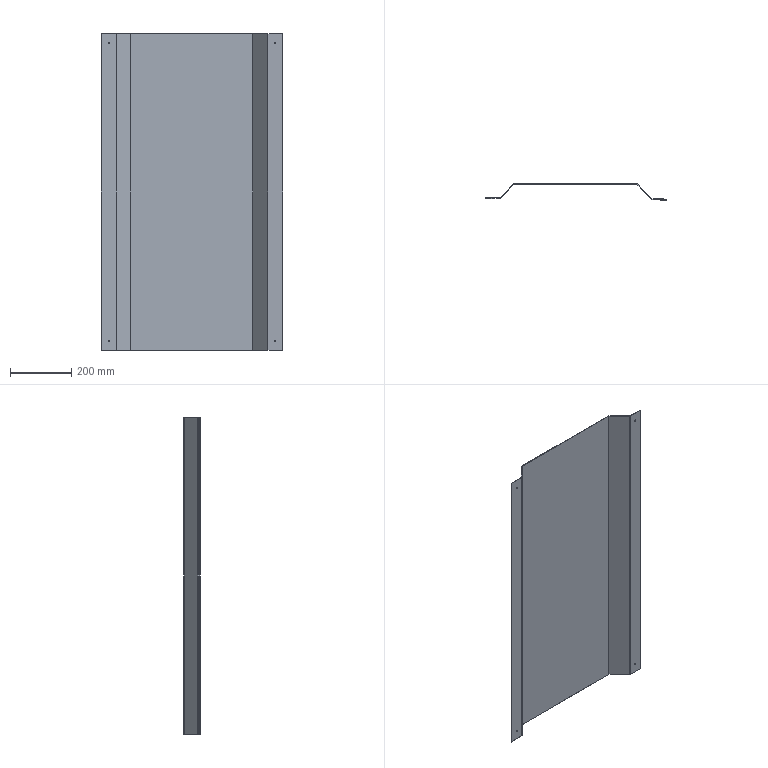Part | STEP file | Assembly TS-S09 | 1 solid | 46 faces | box 590.109 x 52.135 x 1030 mm | volume 1293599 mm3 | plane 30 | cylinder 16 | commonest cylinder face diameters 5 x8 0.4 x4 4.4 x4